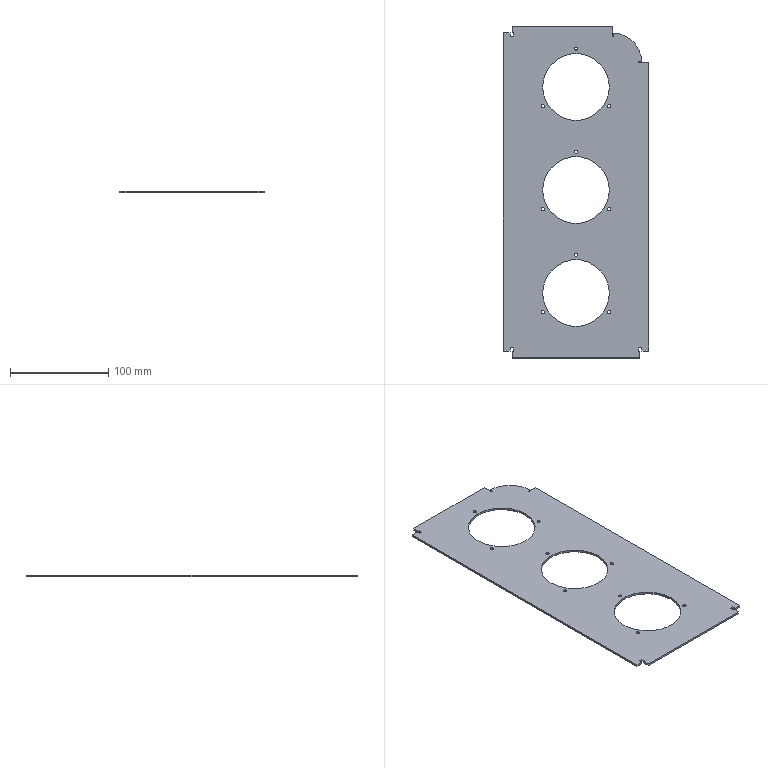Part | STEP file | Oil Pressure Gauge Panel | 1 solid | 55 faces | box 148.239 x 338.239 x 2 mm | volume 76534 mm3 | plane 30 | cylinder 25 | commonest cylinder face diameters 3.2 x18 68 x6 60 x1